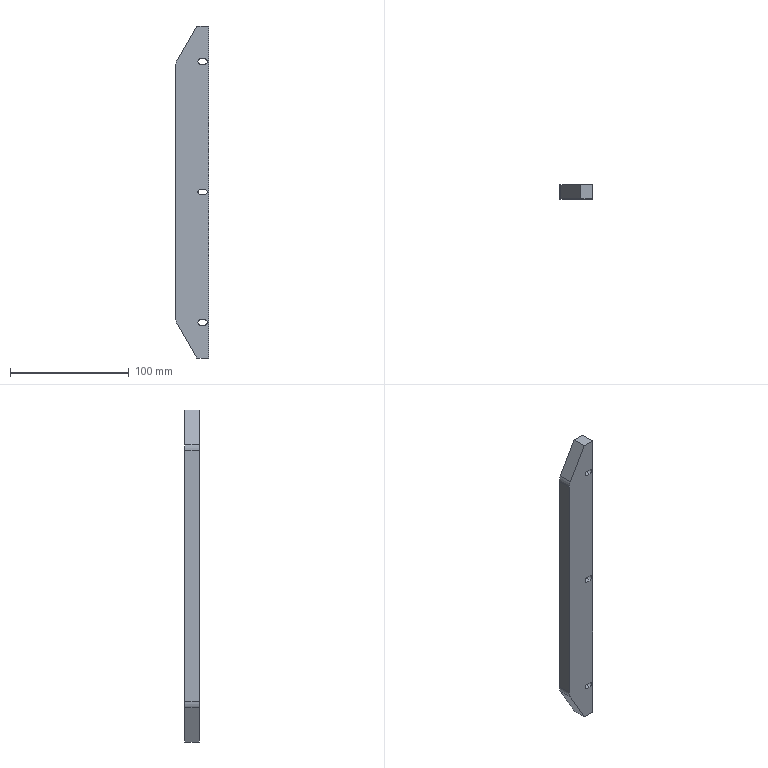Part | STEP file | Tdangtiao-002_デフォルト | 1 solid | 34 faces | box 28 x 12 x 280 mm | volume 85542 mm3 | plane 23 | cylinder 11 | commonest cylinder face diameters 4.5 x6 8.5 x3 20 x2
STEP:
#1=CARTESIAN_POINT('',(9.439,2.,32.25));
#2=VERTEX_POINT('',#1);
#3=CARTESIAN_POINT('',(5.939,2.,32.25));
#4=VERTEX_POINT('',#3);
#5=CARTESIAN_POINT('',(5.939,2.,32.25));
#6=DIRECTION('',(-1.,0.,0.));
#7=VECTOR('',#6,1000.);
#8=LINE('',#5,#7);
#9=EDGE_CURVE('',#2,#4,#8,.T.);
#10=ORIENTED_EDGE('',*,*,#9,.F.);
#11=CARTESIAN_POINT('',(9.439,-6.,32.25));
#12=VERTEX_POINT('',#11);
#13=CARTESIAN_POINT('',(9.439,-274.,32.25));
#14=DIRECTION('',(0.,1.,0.));
#15=VECTOR('',#14,1000.);
#16=LINE('',#13,#15);
#17=EDGE_CURVE('',#12,#2,#16,.T.);
#18=ORIENTED_EDGE('',*,*,#17,.F.);
#19=CARTESIAN_POINT('',(5.939,-6.,32.25));
#20=VERTEX_POINT('',#19);
#21=CARTESIAN_POINT('',(-15.311,-6.,32.25));
#22=DIRECTION('',(1.,0.,0.));
#23=VECTOR('',#22,1000.);
#24=LINE('',#21,#23);
#25=EDGE_CURVE('',#20,#12,#24,.T.);
#26=ORIENTED_EDGE('',*,*,#25,.F.);
#27=CARTESIAN_POINT('',(5.939,-274.,32.25));
#28=DIRECTION('',(0.,1.,0.));
#29=VECTOR('',#28,1000.);
#30=LINE('',#27,#29);
#31=EDGE_CURVE('',#20,#4,#30,.T.);
#32=ORIENTED_EDGE('',*,*,#31,.T.);
#33=EDGE_LOOP('',(#10,#18,#26,#32));
#34=FACE_OUTER_BOUND('',#33,.T.);
#35=CARTESIAN_POINT('',(5.939,-274.,32.25));
#36=DIRECTION('',(0.,0.,1.));
#37=DIRECTION('',(1.,0.,0.));
#38=AXIS2_PLACEMENT_3D('',#35,#36,#37);
#39=PLANE('',#38);
#40=ADVANCED_FACE('',(#34),#39,.F.);
#41=CARTESIAN_POINT('',(9.439,2.,27.75));
#42=VERTEX_POINT('',#41);
#43=CARTESIAN_POINT('',(9.439,2.,30.));
#44=DIRECTION('',(0.,-1.,0.));
#45=DIRECTION('',(0.,0.,1.));
#46=AXIS2_PLACEMENT_3D('',#43,#44,#45);
#47=CIRCLE('',#46,2.25);
#48=EDGE_CURVE('',#42,#2,#47,.T.);
#49=ORIENTED_EDGE('',*,*,#48,.F.);
#50=CARTESIAN_POINT('',(9.439,-6.,27.75));
#51=VERTEX_POINT('',#50);
#52=CARTESIAN_POINT('',(9.439,-274.,27.75));
#53=DIRECTION('',(0.,1.,0.));
#54=VECTOR('',#53,1000.);
#55=LINE('',#52,#54);
#56=EDGE_CURVE('',#51,#42,#55,.T.);
#57=ORIENTED_EDGE('',*,*,#56,.F.);
#58=CARTESIAN_POINT('',(9.439,-6.,30.));
#59=DIRECTION('',(0.,1.,0.));
#60=DIRECTION('',(0.,0.,1.));
#61=AXIS2_PLACEMENT_3D('',#58,#59,#60);
#62=CIRCLE('',#61,2.25);
#63=EDGE_CURVE('',#12,#51,#62,.T.);
#64=ORIENTED_EDGE('',*,*,#63,.F.);
#65=ORIENTED_EDGE('',*,*,#17,.T.);
#66=EDGE_LOOP('',(#49,#57,#64,#65));
#67=FACE_OUTER_BOUND('',#66,.T.);
#68=CARTESIAN_POINT('',(9.439,-274.,30.));
#69=DIRECTION('',(0.,1.,0.));
#70=DIRECTION('',(0.,0.,1.));
#71=AXIS2_PLACEMENT_3D('',#68,#69,#70);
#72=CYLINDRICAL_SURFACE('',#71,2.25);
#73=ADVANCED_FACE('',(#67),#72,.F.);
#74=CARTESIAN_POINT('',(5.939,2.,27.75));
#75=VERTEX_POINT('',#74);
#76=CARTESIAN_POINT('',(5.939,2.,27.75));
#77=DIRECTION('',(1.,0.,0.));
#78=VECTOR('',#77,1000.);
#79=LINE('',#76,#78);
#80=EDGE_CURVE('',#75,#42,#79,.T.);
#81=ORIENTED_EDGE('',*,*,#80,.F.);
#82=CARTESIAN_POINT('',(5.939,-6.,27.75));
#83=VERTEX_POINT('',#82);
#84=CARTESIAN_POINT('',(5.939,-274.,27.75));
#85=DIRECTION('',(0.,1.,0.));
#86=VECTOR('',#85,1000.);
#87=LINE('',#84,#86);
#88=EDGE_CURVE('',#83,#75,#87,.T.);
#89=ORIENTED_EDGE('',*,*,#88,.F.);
#90=CARTESIAN_POINT('',(-15.311,-6.,27.75));
#91=DIRECTION('',(-1.,0.,0.));
#92=VECTOR('',#91,1000.);
#93=LINE('',#90,#92);
#94=EDGE_CURVE('',#51,#83,#93,.T.);
#95=ORIENTED_EDGE('',*,*,#94,.F.);
#96=ORIENTED_EDGE('',*,*,#56,.T.);
#97=EDGE_LOOP('',(#81,#89,#95,#96));
#98=FACE_OUTER_BOUND('',#97,.T.);
#99=CARTESIAN_POINT('',(5.939,-274.,27.75));
#100=DIRECTION('',(0.,0.,-1.));
#101=DIRECTION('',(-1.,0.,0.));
#102=AXIS2_PLACEMENT_3D('',#99,#100,#101);
#103=PLANE('',#102);
#104=ADVANCED_FACE('',(#98),#103,.F.);
#105=CARTESIAN_POINT('',(5.939,2.,30.));
#106=DIRECTION('',(0.,-1.,0.));
#107=DIRECTION('',(0.,0.,1.));
#108=AXIS2_PLACEMENT_3D('',#105,#106,#107);
#109=CIRCLE('',#108,2.25);
#110=EDGE_CURVE('',#4,#75,#109,.T.);
#111=ORIENTED_EDGE('',*,*,#110,.F.);
#112=ORIENTED_EDGE('',*,*,#31,.F.);
#113=CARTESIAN_POINT('',(5.939,-6.,30.));
#114=DIRECTION('',(0.,1.,0.));
#115=DIRECTION('',(0.,0.,1.));
#116=AXIS2_PLACEMENT_3D('',#113,#114,#115);
#117=CIRCLE('',#116,2.25);
#118=EDGE_CURVE('',#83,#20,#117,.T.);
#119=ORIENTED_EDGE('',*,*,#118,.F.);
#120=ORIENTED_EDGE('',*,*,#88,.T.);
#121=EDGE_LOOP('',(#111,#112,#119,#120));
#122=FACE_OUTER_BOUND('',#121,.T.);
#123=CARTESIAN_POINT('',(5.939,-274.,30.));
#124=DIRECTION('',(0.,1.,0.));
#125=DIRECTION('',(0.,0.,1.));
#126=AXIS2_PLACEMENT_3D('',#123,#124,#125);
#127=CYLINDRICAL_SURFACE('',#126,2.25);
#128=ADVANCED_FACE('',(#122),#127,.F.);
#129=CARTESIAN_POINT('',(5.939,2.,142.25));
#130=VERTEX_POINT('',#129);
#131=CARTESIAN_POINT('',(5.939,2.,137.75));
#132=VERTEX_POINT('',#131);
#133=CARTESIAN_POINT('',(5.939,2.,140.));
#134=DIRECTION('',(0.,-1.,0.));
#135=DIRECTION('',(0.,0.,1.));
#136=AXIS2_PLACEMENT_3D('',#133,#134,#135);
#137=CIRCLE('',#136,2.25);
#138=EDGE_CURVE('',#130,#132,#137,.T.);
#139=ORIENTED_EDGE('',*,*,#138,.F.);
#140=CARTESIAN_POINT('',(5.939,-6.,142.25));
#141=VERTEX_POINT('',#140);
#142=CARTESIAN_POINT('',(5.939,-274.,142.25));
#143=DIRECTION('',(0.,1.,0.));
#144=VECTOR('',#143,1000.);
#145=LINE('',#142,#144);
#146=EDGE_CURVE('',#141,#130,#145,.T.);
#147=ORIENTED_EDGE('',*,*,#146,.F.);
#148=CARTESIAN_POINT('',(5.939,-6.,137.75));
#149=VERTEX_POINT('',#148);
#150=CARTESIAN_POINT('',(5.939,-6.,140.));
#151=DIRECTION('',(0.,1.,0.));
#152=DIRECTION('',(0.,0.,1.));
#153=AXIS2_PLACEMENT_3D('',#150,#151,#152);
#154=CIRCLE('',#153,2.25);
#155=EDGE_CURVE('',#149,#141,#154,.T.);
#156=ORIENTED_EDGE('',*,*,#155,.F.);
#157=CARTESIAN_POINT('',(5.939,-274.,137.75));
#158=DIRECTION('',(0.,1.,0.));
#159=VECTOR('',#158,1000.);
#160=LINE('',#157,#159);
#161=EDGE_CURVE('',#149,#132,#160,.T.);
#162=ORIENTED_EDGE('',*,*,#161,.T.);
#163=EDGE_LOOP('',(#139,#147,#156,#162));
#164=FACE_OUTER_BOUND('',#163,.T.);
#165=CARTESIAN_POINT('',(5.939,-274.,140.));
#166=DIRECTION('',(0.,1.,0.));
#167=DIRECTION('',(0.,0.,1.));
#168=AXIS2_PLACEMENT_3D('',#165,#166,#167);
#169=CYLINDRICAL_SURFACE('',#168,2.25);
#170=ADVANCED_FACE('',(#164),#169,.F.);
#171=CARTESIAN_POINT('',(9.439,2.,137.75));
#172=VERTEX_POINT('',#171);
#173=CARTESIAN_POINT('',(5.939,2.,137.75));
#174=DIRECTION('',(1.,0.,0.));
#175=VECTOR('',#174,1000.);
#176=LINE('',#173,#175);
#177=EDGE_CURVE('',#132,#172,#176,.T.);
#178=ORIENTED_EDGE('',*,*,#177,.F.);
#179=ORIENTED_EDGE('',*,*,#161,.F.);
#180=CARTESIAN_POINT('',(9.439,-6.,137.75));
#181=VERTEX_POINT('',#180);
#182=CARTESIAN_POINT('',(-15.311,-6.,137.75));
#183=DIRECTION('',(-1.,0.,0.));
#184=VECTOR('',#183,1000.);
#185=LINE('',#182,#184);
#186=EDGE_CURVE('',#181,#149,#185,.T.);
#187=ORIENTED_EDGE('',*,*,#186,.F.);
#188=CARTESIAN_POINT('',(9.439,-274.,137.75));
#189=DIRECTION('',(0.,1.,0.));
#190=VECTOR('',#189,1000.);
#191=LINE('',#188,#190);
#192=EDGE_CURVE('',#181,#172,#191,.T.);
#193=ORIENTED_EDGE('',*,*,#192,.T.);
#194=EDGE_LOOP('',(#178,#179,#187,#193));
#195=FACE_OUTER_BOUND('',#194,.T.);
#196=CARTESIAN_POINT('',(5.939,-274.,137.75));
#197=DIRECTION('',(0.,0.,-1.));
#198=DIRECTION('',(-1.,0.,0.));
#199=AXIS2_PLACEMENT_3D('',#196,#197,#198);
#200=PLANE('',#199);
#201=ADVANCED_FACE('',(#195),#200,.F.);
#202=CARTESIAN_POINT('',(9.439,2.,142.25));
#203=VERTEX_POINT('',#202);
#204=CARTESIAN_POINT('',(9.439,2.,140.));
#205=DIRECTION('',(0.,-1.,0.));
#206=DIRECTION('',(0.,0.,1.));
#207=AXIS2_PLACEMENT_3D('',#204,#205,#206);
#208=CIRCLE('',#207,2.25);
#209=EDGE_CURVE('',#172,#203,#208,.T.);
#210=ORIENTED_EDGE('',*,*,#209,.F.);
#211=ORIENTED_EDGE('',*,*,#192,.F.);
#212=CARTESIAN_POINT('',(9.439,-6.,142.25));
#213=VERTEX_POINT('',#212);
#214=CARTESIAN_POINT('',(9.439,-6.,140.));
#215=DIRECTION('',(0.,1.,0.));
#216=DIRECTION('',(0.,0.,1.));
#217=AXIS2_PLACEMENT_3D('',#214,#215,#216);
#218=CIRCLE('',#217,2.25);
#219=EDGE_CURVE('',#213,#181,#218,.T.);
#220=ORIENTED_EDGE('',*,*,#219,.F.);
#221=CARTESIAN_POINT('',(9.439,-274.,142.25));
#222=DIRECTION('',(0.,1.,0.));
#223=VECTOR('',#222,1000.);
#224=LINE('',#221,#223);
#225=EDGE_CURVE('',#213,#203,#224,.T.);
#226=ORIENTED_EDGE('',*,*,#225,.T.);
#227=EDGE_LOOP('',(#210,#211,#220,#226));
#228=FACE_OUTER_BOUND('',#227,.T.);
#229=CARTESIAN_POINT('',(9.439,-274.,140.));
#230=DIRECTION('',(0.,1.,0.));
#231=DIRECTION('',(0.,0.,1.));
#232=AXIS2_PLACEMENT_3D('',#229,#230,#231);
#233=CYLINDRICAL_SURFACE('',#232,2.25);
#234=ADVANCED_FACE('',(#228),#233,.F.);
#235=CARTESIAN_POINT('',(5.939,2.,142.25));
#236=DIRECTION('',(-1.,0.,0.));
#237=VECTOR('',#236,1000.);
#238=LINE('',#235,#237);
#239=EDGE_CURVE('',#203,#130,#238,.T.);
#240=ORIENTED_EDGE('',*,*,#239,.F.);
#241=ORIENTED_EDGE('',*,*,#225,.F.);
#242=CARTESIAN_POINT('',(-15.311,-6.,142.25));
#243=DIRECTION('',(1.,0.,0.));
#244=VECTOR('',#243,1000.);
#245=LINE('',#242,#244);
#246=EDGE_CURVE('',#141,#213,#245,.T.);
#247=ORIENTED_EDGE('',*,*,#246,.F.);
#248=ORIENTED_EDGE('',*,*,#146,.T.);
#249=EDGE_LOOP('',(#240,#241,#247,#248));
#250=FACE_OUTER_BOUND('',#249,.T.);
#251=CARTESIAN_POINT('',(5.939,-274.,142.25));
#252=DIRECTION('',(0.,0.,1.));
#253=DIRECTION('',(1.,0.,0.));
#254=AXIS2_PLACEMENT_3D('',#251,#252,#253);
#255=PLANE('',#254);
#256=ADVANCED_FACE('',(#250),#255,.F.);
#257=CARTESIAN_POINT('',(5.939,2.,252.25));
#258=VERTEX_POINT('',#257);
#259=CARTESIAN_POINT('',(5.939,2.,247.75));
#260=VERTEX_POINT('',#259);
#261=CARTESIAN_POINT('',(5.939,2.,250.));
#262=DIRECTION('',(0.,-1.,0.));
#263=DIRECTION('',(0.,0.,1.));
#264=AXIS2_PLACEMENT_3D('',#261,#262,#263);
#265=CIRCLE('',#264,2.25);
#266=EDGE_CURVE('',#258,#260,#265,.T.);
#267=ORIENTED_EDGE('',*,*,#266,.F.);
#268=CARTESIAN_POINT('',(5.939,-6.,252.25));
#269=VERTEX_POINT('',#268);
#270=CARTESIAN_POINT('',(5.939,-274.,252.25));
#271=DIRECTION('',(0.,1.,0.));
#272=VECTOR('',#271,1000.);
#273=LINE('',#270,#272);
#274=EDGE_CURVE('',#269,#258,#273,.T.);
#275=ORIENTED_EDGE('',*,*,#274,.F.);
#276=CARTESIAN_POINT('',(5.939,-6.,247.75));
#277=VERTEX_POINT('',#276);
#278=CARTESIAN_POINT('',(5.939,-6.,250.));
#279=DIRECTION('',(0.,1.,0.));
#280=DIRECTION('',(0.,0.,1.));
#281=AXIS2_PLACEMENT_3D('',#278,#279,#280);
#282=CIRCLE('',#281,2.25);
#283=EDGE_CURVE('',#277,#269,#282,.T.);
#284=ORIENTED_EDGE('',*,*,#283,.F.);
#285=CARTESIAN_POINT('',(5.939,-274.,247.75));
#286=DIRECTION('',(0.,1.,0.));
#287=VECTOR('',#286,1000.);
#288=LINE('',#285,#287);
#289=EDGE_CURVE('',#277,#260,#288,.T.);
#290=ORIENTED_EDGE('',*,*,#289,.T.);
#291=EDGE_LOOP('',(#267,#275,#284,#290));
#292=FACE_OUTER_BOUND('',#291,.T.);
#293=CARTESIAN_POINT('',(5.939,-274.,250.));
#294=DIRECTION('',(0.,1.,0.));
#295=DIRECTION('',(0.,0.,1.));
#296=AXIS2_PLACEMENT_3D('',#293,#294,#295);
#297=CYLINDRICAL_SURFACE('',#296,2.25);
#298=ADVANCED_FACE('',(#292),#297,.F.);
#299=CARTESIAN_POINT('',(9.439,2.,247.75));
#300=VERTEX_POINT('',#299);
#301=CARTESIAN_POINT('',(5.939,2.,247.75));
#302=DIRECTION('',(1.,0.,0.));
#303=VECTOR('',#302,1000.);
#304=LINE('',#301,#303);
#305=EDGE_CURVE('',#260,#300,#304,.T.);
#306=ORIENTED_EDGE('',*,*,#305,.F.);
#307=ORIENTED_EDGE('',*,*,#289,.F.);
#308=CARTESIAN_POINT('',(9.439,-6.,247.75));
#309=VERTEX_POINT('',#308);
#310=CARTESIAN_POINT('',(-15.311,-6.,247.75));
#311=DIRECTION('',(-1.,0.,0.));
#312=VECTOR('',#311,1000.);
#313=LINE('',#310,#312);
#314=EDGE_CURVE('',#309,#277,#313,.T.);
#315=ORIENTED_EDGE('',*,*,#314,.F.);
#316=CARTESIAN_POINT('',(9.439,-274.,247.75));
#317=DIRECTION('',(0.,1.,0.));
#318=VECTOR('',#317,1000.);
#319=LINE('',#316,#318);
#320=EDGE_CURVE('',#309,#300,#319,.T.);
#321=ORIENTED_EDGE('',*,*,#320,.T.);
#322=EDGE_LOOP('',(#306,#307,#315,#321));
#323=FACE_OUTER_BOUND('',#322,.T.);
#324=CARTESIAN_POINT('',(5.939,-274.,247.75));
#325=DIRECTION('',(0.,0.,-1.));
#326=DIRECTION('',(-1.,0.,0.));
#327=AXIS2_PLACEMENT_3D('',#324,#325,#326);
#328=PLANE('',#327);
#329=ADVANCED_FACE('',(#323),#328,.F.);
#330=CARTESIAN_POINT('',(9.439,2.,252.25));
#331=VERTEX_POINT('',#330);
#332=CARTESIAN_POINT('',(9.439,2.,250.));
#333=DIRECTION('',(0.,-1.,0.));
#334=DIRECTION('',(0.,0.,1.));
#335=AXIS2_PLACEMENT_3D('',#332,#333,#334);
#336=CIRCLE('',#335,2.25);
#337=EDGE_CURVE('',#300,#331,#336,.T.);
#338=ORIENTED_EDGE('',*,*,#337,.F.);
#339=ORIENTED_EDGE('',*,*,#320,.F.);
#340=CARTESIAN_POINT('',(9.439,-6.,252.25));
#341=VERTEX_POINT('',#340);
#342=CARTESIAN_POINT('',(9.439,-6.,250.));
#343=DIRECTION('',(0.,1.,0.));
#344=DIRECTION('',(0.,0.,1.));
#345=AXIS2_PLACEMENT_3D('',#342,#343,#344);
#346=CIRCLE('',#345,2.25);
#347=EDGE_CURVE('',#341,#309,#346,.T.);
#348=ORIENTED_EDGE('',*,*,#347,.F.);
#349=CARTESIAN_POINT('',(9.439,-274.,252.25));
#350=DIRECTION('',(0.,1.,0.));
#351=VECTOR('',#350,1000.);
#352=LINE('',#349,#351);
#353=EDGE_CURVE('',#341,#331,#352,.T.);
#354=ORIENTED_EDGE('',*,*,#353,.T.);
#355=EDGE_LOOP('',(#338,#339,#348,#354));
#356=FACE_OUTER_BOUND('',#355,.T.);
#357=CARTESIAN_POINT('',(9.439,-274.,250.));
#358=DIRECTION('',(0.,1.,0.));
#359=DIRECTION('',(0.,0.,1.));
#360=AXIS2_PLACEMENT_3D('',#357,#358,#359);
#361=CYLINDRICAL_SURFACE('',#360,2.25);
#362=ADVANCED_FACE('',(#356),#361,.F.);
#363=CARTESIAN_POINT('',(5.939,2.,252.25));
#364=DIRECTION('',(-1.,0.,0.));
#365=VECTOR('',#364,1000.);
#366=LINE('',#363,#365);
#367=EDGE_CURVE('',#331,#258,#366,.T.);
#368=ORIENTED_EDGE('',*,*,#367,.F.);
#369=ORIENTED_EDGE('',*,*,#353,.F.);
#370=CARTESIAN_POINT('',(-15.311,-6.,252.25));
#371=DIRECTION('',(1.,0.,0.));
#372=VECTOR('',#371,1000.);
#373=LINE('',#370,#372);
#374=EDGE_CURVE('',#269,#341,#373,.T.);
#375=ORIENTED_EDGE('',*,*,#374,.F.);
#376=ORIENTED_EDGE('',*,*,#274,.T.);
#377=EDGE_LOOP('',(#368,#369,#375,#376));
#378=FACE_OUTER_BOUND('',#377,.T.);
#379=CARTESIAN_POINT('',(5.939,-274.,252.25));
#380=DIRECTION('',(0.,0.,1.));
#381=DIRECTION('',(1.,0.,0.));
#382=AXIS2_PLACEMENT_3D('',#379,#380,#381);
#383=PLANE('',#382);
#384=ADVANCED_FACE('',(#378),#383,.F.);
#385=CARTESIAN_POINT('',(12.689,2.,34.25));
#386=VERTEX_POINT('',#385);
#387=CARTESIAN_POINT('',(12.689,2.,25.75));
#388=VERTEX_POINT('',#387);
#389=CARTESIAN_POINT('',(12.689,2.,280.));
#390=DIRECTION('',(0.,0.,-1.));
#391=VECTOR('',#390,1000.);
#392=LINE('',#389,#391);
#393=EDGE_CURVE('',#386,#388,#392,.T.);
#394=ORIENTED_EDGE('',*,*,#393,.F.);
#395=CARTESIAN_POINT('',(12.689,6.,34.25));
#396=VERTEX_POINT('',#395);
#397=CARTESIAN_POINT('',(12.689,6.,34.25));
#398=DIRECTION('',(0.,1.,0.));
#399=VECTOR('',#398,1000.);
#400=LINE('',#397,#399);
#401=EDGE_CURVE('',#386,#396,#400,.T.);
#402=ORIENTED_EDGE('',*,*,#401,.T.);
#403=CARTESIAN_POINT('',(12.689,6.,135.75));
#404=VERTEX_POINT('',#403);
#405=CARTESIAN_POINT('',(12.689,6.,280.));
#406=DIRECTION('',(0.,0.,-1.));
#407=VECTOR('',#406,1000.);
#408=LINE('',#405,#407);
#409=EDGE_CURVE('',#404,#396,#408,.T.);
#410=ORIENTED_EDGE('',*,*,#409,.F.);
#411=CARTESIAN_POINT('',(12.689,2.,135.75));
#412=VERTEX_POINT('',#411);
#413=CARTESIAN_POINT('',(12.689,6.,135.75));
#414=DIRECTION('',(0.,-1.,0.));
#415=VECTOR('',#414,1000.);
#416=LINE('',#413,#415);
#417=EDGE_CURVE('',#404,#412,#416,.T.);
#418=ORIENTED_EDGE('',*,*,#417,.T.);
#419=CARTESIAN_POINT('',(12.689,2.,144.25));
#420=VERTEX_POINT('',#419);
#421=CARTESIAN_POINT('',(12.689,2.,280.));
#422=DIRECTION('',(0.,0.,-1.));
#423=VECTOR('',#422,1000.);
#424=LINE('',#421,#423);
#425=EDGE_CURVE('',#420,#412,#424,.T.);
#426=ORIENTED_EDGE('',*,*,#425,.F.);
#427=CARTESIAN_POINT('',(12.689,6.,144.25));
#428=VERTEX_POINT('',#427);
#429=CARTESIAN_POINT('',(12.689,6.,144.25));
#430=DIRECTION('',(0.,1.,0.));
#431=VECTOR('',#430,1000.);
#432=LINE('',#429,#431);
#433=EDGE_CURVE('',#420,#428,#432,.T.);
#434=ORIENTED_EDGE('',*,*,#433,.T.);
#435=CARTESIAN_POINT('',(12.689,6.,245.75));
#436=VERTEX_POINT('',#435);
#437=CARTESIAN_POINT('',(12.689,6.,280.));
#438=DIRECTION('',(0.,0.,-1.));
#439=VECTOR('',#438,1000.);
#440=LINE('',#437,#439);
#441=EDGE_CURVE('',#436,#428,#440,.T.);
#442=ORIENTED_EDGE('',*,*,#441,.F.);
#443=CARTESIAN_POINT('',(12.689,2.,245.75));
#444=VERTEX_POINT('',#443);
#445=CARTESIAN_POINT('',(12.689,6.,245.75));
#446=DIRECTION('',(0.,-1.,0.));
#447=VECTOR('',#446,1000.);
#448=LINE('',#445,#447);
#449=EDGE_CURVE('',#436,#444,#448,.T.);
#450=ORIENTED_EDGE('',*,*,#449,.T.);
#451=CARTESIAN_POINT('',(12.689,2.,254.25));
#452=VERTEX_POINT('',#451);
#453=CARTESIAN_POINT('',(12.689,2.,280.));
#454=DIRECTION('',(0.,0.,-1.));
#455=VECTOR('',#454,1000.);
#456=LINE('',#453,#455);
#457=EDGE_CURVE('',#452,#444,#456,.T.);
#458=ORIENTED_EDGE('',*,*,#457,.F.);
#459=CARTESIAN_POINT('',(12.689,6.,254.25));
#460=VERTEX_POINT('',#459);
#461=CARTESIAN_POINT('',(12.689,6.,254.25));
#462=DIRECTION('',(0.,1.,0.));
#463=VECTOR('',#462,1000.);
#464=LINE('',#461,#463);
#465=EDGE_CURVE('',#452,#460,#464,.T.);
#466=ORIENTED_EDGE('',*,*,#465,.T.);
#467=CARTESIAN_POINT('',(12.689,6.,280.));
#468=VERTEX_POINT('',#467);
#469=CARTESIAN_POINT('',(12.689,6.,280.));
#470=DIRECTION('',(0.,0.,-1.));
#471=VECTOR('',#470,1000.);
#472=LINE('',#469,#471);
#473=EDGE_CURVE('',#468,#460,#472,.T.);
#474=ORIENTED_EDGE('',*,*,#473,.F.);
#475=CARTESIAN_POINT('',(12.689,-6.,280.));
#476=VERTEX_POINT('',#475);
#477=CARTESIAN_POINT('',(12.689,6.,280.));
#478=DIRECTION('',(0.,1.,0.));
#479=VECTOR('',#478,1000.);
#480=LINE('',#477,#479);
#481=EDGE_CURVE('',#476,#468,#480,.T.);
#482=ORIENTED_EDGE('',*,*,#481,.F.);
#483=CARTESIAN_POINT('',(12.689,-6.,0.));
#484=VERTEX_POINT('',#483);
#485=CARTESIAN_POINT('',(12.689,-6.,280.));
#486=DIRECTION('',(0.,0.,-1.));
#487=VECTOR('',#486,1000.);
#488=LINE('',#485,#487);
#489=EDGE_CURVE('',#476,#484,#488,.T.);
#490=ORIENTED_EDGE('',*,*,#489,.T.);
#491=CARTESIAN_POINT('',(12.689,6.,0.));
#492=VERTEX_POINT('',#491);
#493=CARTESIAN_POINT('',(12.689,6.,0.));
#494=DIRECTION('',(0.,1.,0.));
#495=VECTOR('',#494,1000.);
#496=LINE('',#493,#495);
#497=EDGE_CURVE('',#484,#492,#496,.T.);
#498=ORIENTED_EDGE('',*,*,#497,.T.);
#499=CARTESIAN_POINT('',(12.689,6.,25.75));
#500=VERTEX_POINT('',#499);
#501=CARTESIAN_POINT('',(12.689,6.,280.));
#502=DIRECTION('',(0.,0.,-1.));
#503=VECTOR('',#502,1000.);
#504=LINE('',#501,#503);
#505=EDGE_CURVE('',#500,#492,#504,.T.);
#506=ORIENTED_EDGE('',*,*,#505,.F.);
#507=CARTESIAN_POINT('',(12.689,6.,25.75));
#508=DIRECTION('',(0.,-1.,0.));
#509=VECTOR('',#508,1000.);
#510=LINE('',#507,#509);
#511=EDGE_CURVE('',#500,#388,#510,.T.);
#512=ORIENTED_EDGE('',*,*,#511,.T.);
#513=EDGE_LOOP('',(#394,#402,#410,#418,#426,#434,#442,#450,#458,#466,#474,#482,#490,#498,#506,#512));
#514=FACE_OUTER_BOUND('',#513,.T.);
#515=CARTESIAN_POINT('',(12.689,6.,280.));
#516=DIRECTION('',(-1.,0.,0.));
#517=DIRECTION('',(0.,-1.,0.));
#518=AXIS2_PLACEMENT_3D('',#515,#516,#517);
#519=PLANE('',#518);
#520=ADVANCED_FACE('',(#514),#519,.F.);
#521=CARTESIAN_POINT('',(-15.311,6.,246.144));
#522=VERTEX_POINT('',#521);
#523=CARTESIAN_POINT('',(-15.311,6.,33.856));
#524=VERTEX_POINT('',#523);
#525=CARTESIAN_POINT('',(-15.311,6.,280.));
#526=DIRECTION('',(0.,0.,-1.));
#527=VECTOR('',#526,1000.);
#528=LINE('',#525,#527);
#529=EDGE_CURVE('',#522,#524,#528,.T.);
#530=ORIENTED_EDGE('',*,*,#529,.F.);
#531=CARTESIAN_POINT('',(-13.971,6.,251.144));
#532=VERTEX_POINT('',#531);
#533=CARTESIAN_POINT('',(-5.311,6.,246.144));
#534=DIRECTION('',(0.,1.,0.));
#535=DIRECTION('',(0.,0.,-1.));
#536=AXIS2_PLACEMENT_3D('',#533,#534,#535);
#537=CIRCLE('',#536,10.);
#538=EDGE_CURVE('',#522,#532,#537,.T.);
#539=ORIENTED_EDGE('',*,*,#538,.T.);
#540=CARTESIAN_POINT('',(2.689,6.,280.));
#541=VERTEX_POINT('',#540);
#542=CARTESIAN_POINT('',(2.689,6.,280.));
#543=DIRECTION('',(-0.5,0.,-0.866));
#544=VECTOR('',#543,1000.);
#545=LINE('',#542,#544);
#546=EDGE_CURVE('',#541,#532,#545,.T.);
#547=ORIENTED_EDGE('',*,*,#546,.F.);
#548=CARTESIAN_POINT('',(-15.311,6.,280.));
#549=DIRECTION('',(-1.,0.,0.));
#550=VECTOR('',#549,1000.);
#551=LINE('',#548,#550);
#552=EDGE_CURVE('',#468,#541,#551,.T.);
#553=ORIENTED_EDGE('',*,*,#552,.F.);
#554=ORIENTED_EDGE('',*,*,#473,.T.);
#555=CARTESIAN_POINT('',(5.939,6.,254.25));
#556=VERTEX_POINT('',#555);
#557=CARTESIAN_POINT('',(23.402,6.,254.25));
#558=DIRECTION('',(1.,0.,0.));
#559=VECTOR('',#558,1000.);
#560=LINE('',#557,#559);
#561=EDGE_CURVE('',#556,#460,#560,.T.);
#562=ORIENTED_EDGE('',*,*,#561,.F.);
#563=CARTESIAN_POINT('',(5.939,6.,245.75));
#564=VERTEX_POINT('',#563);
#565=CARTESIAN_POINT('',(5.939,6.,250.));
#566=DIRECTION('',(0.,1.,0.));
#567=DIRECTION('',(0.,0.,1.));
#568=AXIS2_PLACEMENT_3D('',#565,#566,#567);
#569=CIRCLE('',#568,4.25);
#570=EDGE_CURVE('',#564,#556,#569,.T.);
#571=ORIENTED_EDGE('',*,*,#570,.F.);
#572=CARTESIAN_POINT('',(9.439,6.,245.75));
#573=DIRECTION('',(-1.,0.,0.));
#574=VECTOR('',#573,1000.);
#575=LINE('',#572,#574);
#576=EDGE_CURVE('',#436,#564,#575,.T.);
#577=ORIENTED_EDGE('',*,*,#576,.F.);
#578=ORIENTED_EDGE('',*,*,#441,.T.);
#579=CARTESIAN_POINT('',(5.939,6.,144.25));
#580=VERTEX_POINT('',#579);
#581=CARTESIAN_POINT('',(23.402,6.,144.25));
#582=DIRECTION('',(1.,0.,0.));
#583=VECTOR('',#582,1000.);
#584=LINE('',#581,#583);
#585=EDGE_CURVE('',#580,#428,#584,.T.);
#586=ORIENTED_EDGE('',*,*,#585,.F.);
#587=CARTESIAN_POINT('',(5.939,6.,135.75));
#588=VERTEX_POINT('',#587);
#589=CARTESIAN_POINT('',(5.939,6.,140.));
#590=DIRECTION('',(0.,1.,0.));
#591=DIRECTION('',(0.,0.,1.));
#592=AXIS2_PLACEMENT_3D('',#589,#590,#591);
#593=CIRCLE('',#592,4.25);
#594=EDGE_CURVE('',#588,#580,#593,.T.);
#595=ORIENTED_EDGE('',*,*,#594,.F.);
#596=CARTESIAN_POINT('',(9.439,6.,135.75));
#597=DIRECTION('',(-1.,0.,0.));
#598=VECTOR('',#597,1000.);
#599=LINE('',#596,#598);
#600=EDGE_CURVE('',#404,#588,#599,.T.);
#601=ORIENTED_EDGE('',*,*,#600,.F.);
#602=ORIENTED_EDGE('',*,*,#409,.T.);
#603=CARTESIAN_POINT('',(5.939,6.,34.25));
#604=VERTEX_POINT('',#603);
#605=CARTESIAN_POINT('',(23.402,6.,34.25));
#606=DIRECTION('',(1.,0.,0.));
#607=VECTOR('',#606,1000.);
#608=LINE('',#605,#607);
#609=EDGE_CURVE('',#604,#396,#608,.T.);
#610=ORIENTED_EDGE('',*,*,#609,.F.);
#611=CARTESIAN_POINT('',(5.939,6.,25.75));
#612=VERTEX_POINT('',#611);
#613=CARTESIAN_POINT('',(5.939,6.,30.));
#614=DIRECTION('',(0.,1.,0.));
#615=DIRECTION('',(0.,0.,1.));
#616=AXIS2_PLACEMENT_3D('',#613,#614,#615);
#617=CIRCLE('',#616,4.25);
#618=EDGE_CURVE('',#612,#604,#617,.T.);
#619=ORIENTED_EDGE('',*,*,#618,.F.);
#620=CARTESIAN_POINT('',(9.439,6.,25.75));
#621=DIRECTION('',(-1.,0.,0.));
#622=VECTOR('',#621,1000.);
#623=LINE('',#620,#622);
#624=EDGE_CURVE('',#500,#612,#623,.T.);
#625=ORIENTED_EDGE('',*,*,#624,.F.);
#626=ORIENTED_EDGE('',*,*,#505,.T.);
#627=CARTESIAN_POINT('',(2.689,6.,0.));
#628=VERTEX_POINT('',#627);
#629=CARTESIAN_POINT('',(-15.311,6.,0.));
#630=DIRECTION('',(-1.,0.,0.));
#631=VECTOR('',#630,1000.);
#632=LINE('',#629,#631);
#633=EDGE_CURVE('',#492,#628,#632,.T.);
#634=ORIENTED_EDGE('',*,*,#633,.T.);
#635=CARTESIAN_POINT('',(-13.971,6.,28.856));
#636=VERTEX_POINT('',#635);
#637=CARTESIAN_POINT('',(2.689,6.,0.));
#638=DIRECTION('',(0.5,0.,-0.866));
#639=VECTOR('',#638,1000.);
#640=LINE('',#637,#639);
#641=EDGE_CURVE('',#636,#628,#640,.T.);
#642=ORIENTED_EDGE('',*,*,#641,.F.);
#643=CARTESIAN_POINT('',(-5.311,6.,33.856));
#644=DIRECTION('',(0.,1.,0.));
#645=DIRECTION('',(0.,0.,-1.));
#646=AXIS2_PLACEMENT_3D('',#643,#644,#645);
#647=CIRCLE('',#646,10.);
#648=EDGE_CURVE('',#636,#524,#647,.T.);
#649=ORIENTED_EDGE('',*,*,#648,.T.);
#650=EDGE_LOOP('',(#530,#539,#547,#553,#554,#562,#571,#577,#578,#586,#595,#601,#602,#610,#619,#625,#626,#634,#642,#649));
#651=FACE_OUTER_BOUND('',#650,.T.);
#652=CARTESIAN_POINT('',(-15.311,6.,280.));
#653=DIRECTION('',(0.,-1.,0.));
#654=DIRECTION('',(0.,0.,-1.));
#655=AXIS2_PLACEMENT_3D('',#652,#653,#654);
#656=PLANE('',#655);
#657=ADVANCED_FACE('',(#651),#656,.F.);
#658=CARTESIAN_POINT('',(-15.311,-6.,246.144));
#659=VERTEX_POINT('',#658);
#660=CARTESIAN_POINT('',(-15.311,-6.,33.856));
#661=VERTEX_POINT('',#660);
#662=CARTESIAN_POINT('',(-15.311,-6.,280.));
#663=DIRECTION('',(0.,0.,-1.));
#664=VECTOR('',#663,1000.);
#665=LINE('',#662,#664);
#666=EDGE_CURVE('',#659,#661,#665,.T.);
#667=ORIENTED_EDGE('',*,*,#666,.F.);
#668=CARTESIAN_POINT('',(-15.311,6.,246.144));
#669=DIRECTION('',(0.,1.,0.));
#670=VECTOR('',#669,1000.);
#671=LINE('',#668,#670);
#672=EDGE_CURVE('',#659,#522,#671,.T.);
#673=ORIENTED_EDGE('',*,*,#672,.T.);
#674=ORIENTED_EDGE('',*,*,#529,.T.);
#675=CARTESIAN_POINT('',(-15.311,6.,33.856));
#676=DIRECTION('',(0.,-1.,0.));
#677=VECTOR('',#676,1000.);
#678=LINE('',#675,#677);
#679=EDGE_CURVE('',#524,#661,#678,.T.);
#680=ORIENTED_EDGE('',*,*,#679,.T.);
#681=EDGE_LOOP('',(#667,#673,#674,#680));
#682=FACE_OUTER_BOUND('',#681,.T.);
#683=CARTESIAN_POINT('',(-15.311,6.,280.));
#684=DIRECTION('',(1.,0.,0.));
#685=DIRECTION('',(0.,1.,0.));
#686=AXIS2_PLACEMENT_3D('',#683,#684,#685);
#687=PLANE('',#686);
#688=ADVANCED_FACE('',(#682),#687,.F.);
#689=ORIENTED_EDGE('',*,*,#186,.T.);
#690=ORIENTED_EDGE('',*,*,#155,.T.);
#691=ORIENTED_EDGE('',*,*,#246,.T.);
#692=ORIENTED_EDGE('',*,*,#219,.T.);
#693=EDGE_LOOP('',(#689,#690,#691,#692));
#694=FACE_BOUND('',#693,.T.);
#695=ORIENTED_EDGE('',*,*,#314,.T.);
#696=ORIENTED_EDGE('',*,*,#283,.T.);
#697=ORIENTED_EDGE('',*,*,#374,.T.);
#698=ORIENTED_EDGE('',*,*,#347,.T.);
#699=EDGE_LOOP('',(#695,#696,#697,#698));
#700=FACE_BOUND('',#699,.T.);
#701=CARTESIAN_POINT('',(2.689,-6.,280.));
#702=VERTEX_POINT('',#701);
#703=CARTESIAN_POINT('',(-13.971,-6.,251.144));
#704=VERTEX_POINT('',#703);
#705=CARTESIAN_POINT('',(-1.811,-6.,272.206));
#706=DIRECTION('',(-0.5,0.,-0.866));
#707=VECTOR('',#706,1000.);
#708=LINE('',#705,#707);
#709=EDGE_CURVE('',#702,#704,#708,.T.);
#710=ORIENTED_EDGE('',*,*,#709,.T.);
#711=CARTESIAN_POINT('',(-5.311,-6.,246.144));
#712=DIRECTION('',(0.,-1.,0.));
#713=DIRECTION('',(0.,0.,1.));
#714=AXIS2_PLACEMENT_3D('',#711,#712,#713);
#715=CIRCLE('',#714,10.);
#716=EDGE_CURVE('',#704,#659,#715,.T.);
#717=ORIENTED_EDGE('',*,*,#716,.T.);
#718=ORIENTED_EDGE('',*,*,#666,.T.);
#719=CARTESIAN_POINT('',(-13.971,-6.,28.856));
#720=VERTEX_POINT('',#719);
#721=CARTESIAN_POINT('',(-5.311,-6.,33.856));
#722=DIRECTION('',(0.,-1.,0.));
#723=DIRECTION('',(0.,0.,1.));
#724=AXIS2_PLACEMENT_3D('',#721,#722,#723);
#725=CIRCLE('',#724,10.);
#726=EDGE_CURVE('',#661,#720,#725,.T.);
#727=ORIENTED_EDGE('',*,*,#726,.T.);
#728=CARTESIAN_POINT('',(2.689,-6.,0.));
#729=VERTEX_POINT('',#728);
#730=CARTESIAN_POINT('',(-123.055,-6.,217.794));
#731=DIRECTION('',(0.5,0.,-0.866));
#732=VECTOR('',#731,1000.);
#733=LINE('',#730,#732);
#734=EDGE_CURVE('',#720,#729,#733,.T.);
#735=ORIENTED_EDGE('',*,*,#734,.T.);
#736=CARTESIAN_POINT('',(-15.311,-6.,0.));
#737=DIRECTION('',(1.,0.,0.));
#738=VECTOR('',#737,1000.);
#739=LINE('',#736,#738);
#740=EDGE_CURVE('',#729,#484,#739,.T.);
#741=ORIENTED_EDGE('',*,*,#740,.T.);
#742=ORIENTED_EDGE('',*,*,#489,.F.);
#743=CARTESIAN_POINT('',(-15.311,-6.,280.));
#744=DIRECTION('',(1.,0.,0.));
#745=VECTOR('',#744,1000.);
#746=LINE('',#743,#745);
#747=EDGE_CURVE('',#702,#476,#746,.T.);
#748=ORIENTED_EDGE('',*,*,#747,.F.);
#749=EDGE_LOOP('',(#710,#717,#718,#727,#735,#741,#742,#748));
#750=FACE_OUTER_BOUND('',#749,.T.);
#751=ORIENTED_EDGE('',*,*,#118,.T.);
#752=ORIENTED_EDGE('',*,*,#25,.T.);
#753=ORIENTED_EDGE('',*,*,#63,.T.);
#754=ORIENTED_EDGE('',*,*,#94,.T.);
#755=EDGE_LOOP('',(#751,#752,#753,#754));
#756=FACE_BOUND('',#755,.T.);
#757=CARTESIAN_POINT('',(-15.311,-6.,280.));
#758=DIRECTION('',(0.,1.,0.));
#759=DIRECTION('',(0.,0.,1.));
#760=AXIS2_PLACEMENT_3D('',#757,#758,#759);
#761=PLANE('',#760);
#762=ADVANCED_FACE('',(#694,#700,#750,#756),#761,.F.);
#763=CARTESIAN_POINT('',(2.689,0.,280.));
#764=DIRECTION('',(0.,1.,0.));
#765=VECTOR('',#764,1000.);
#766=LINE('',#763,#765);
#767=EDGE_CURVE('',#702,#541,#766,.T.);
#768=ORIENTED_EDGE('',*,*,#767,.F.);
#769=ORIENTED_EDGE('',*,*,#747,.T.);
#770=ORIENTED_EDGE('',*,*,#481,.T.);
#771=ORIENTED_EDGE('',*,*,#552,.T.);
#772=EDGE_LOOP('',(#768,#769,#770,#771));
#773=FACE_OUTER_BOUND('',#772,.T.);
#774=CARTESIAN_POINT('',(0.,0.,280.));
#775=DIRECTION('',(0.,0.,1.));
#776=DIRECTION('',(1.,0.,0.));
#777=AXIS2_PLACEMENT_3D('',#774,#775,#776);
#778=PLANE('',#777);
#779=ADVANCED_FACE('',(#773),#778,.T.);
#780=ORIENTED_EDGE('',*,*,#740,.F.);
#781=CARTESIAN_POINT('',(2.689,0.,0.));
#782=DIRECTION('',(0.,1.,0.));
#783=VECTOR('',#782,1000.);
#784=LINE('',#781,#783);
#785=EDGE_CURVE('',#729,#628,#784,.T.);
#786=ORIENTED_EDGE('',*,*,#785,.T.);
#787=ORIENTED_EDGE('',*,*,#633,.F.);
#788=ORIENTED_EDGE('',*,*,#497,.F.);
#789=EDGE_LOOP('',(#780,#786,#787,#788));
#790=FACE_OUTER_BOUND('',#789,.T.);
#791=CARTESIAN_POINT('',(0.,0.,0.));
#792=DIRECTION('',(0.,0.,1.));
#793=DIRECTION('',(1.,0.,0.));
#794=AXIS2_PLACEMENT_3D('',#791,#792,#793);
#795=PLANE('',#794);
#796=ADVANCED_FACE('',(#790),#795,.F.);
#797=CARTESIAN_POINT('',(5.939,2.,254.25));
#798=VERTEX_POINT('',#797);
#799=CARTESIAN_POINT('',(5.939,2.,254.25));
#800=DIRECTION('',(1.,0.,0.));
#801=VECTOR('',#800,1000.);
#802=LINE('',#799,#801);
#803=EDGE_CURVE('',#798,#452,#802,.T.);
#804=ORIENTED_EDGE('',*,*,#803,.F.);
#805=CARTESIAN_POINT('',(5.939,2.,254.25));
#806=DIRECTION('',(0.,1.,0.));
#807=VECTOR('',#806,1000.);
#808=LINE('',#805,#807);
#809=EDGE_CURVE('',#798,#556,#808,.T.);
#810=ORIENTED_EDGE('',*,*,#809,.T.);
#811=ORIENTED_EDGE('',*,*,#561,.T.);
#812=ORIENTED_EDGE('',*,*,#465,.F.);
#813=EDGE_LOOP('',(#804,#810,#811,#812));
#814=FACE_OUTER_BOUND('',#813,.T.);
#815=CARTESIAN_POINT('',(23.402,2.,254.25));
#816=DIRECTION('',(0.,0.,1.));
#817=DIRECTION('',(1.,0.,0.));
#818=AXIS2_PLACEMENT_3D('',#815,#816,#817);
#819=PLANE('',#818);
#820=ADVANCED_FACE('',(#814),#819,.F.);
#821=ORIENTED_EDGE('',*,*,#576,.T.);
#822=CARTESIAN_POINT('',(5.939,2.,245.75));
#823=VERTEX_POINT('',#822);
#824=CARTESIAN_POINT('',(5.939,2.,245.75));
#825=DIRECTION('',(0.,1.,0.));
#826=VECTOR('',#825,1000.);
#827=LINE('',#824,#826);
#828=EDGE_CURVE('',#823,#564,#827,.T.);
#829=ORIENTED_EDGE('',*,*,#828,.F.);
#830=CARTESIAN_POINT('',(9.439,2.,245.75));
#831=DIRECTION('',(-1.,0.,0.));
#832=VECTOR('',#831,1000.);
#833=LINE('',#830,#832);
#834=EDGE_CURVE('',#444,#823,#833,.T.);
#835=ORIENTED_EDGE('',*,*,#834,.F.);
#836=ORIENTED_EDGE('',*,*,#449,.F.);
#837=EDGE_LOOP('',(#821,#829,#835,#836));
#838=FACE_OUTER_BOUND('',#837,.T.);
#839=CARTESIAN_POINT('',(9.439,2.,245.75));
#840=DIRECTION('',(0.,0.,-1.));
#841=DIRECTION('',(-1.,0.,0.));
#842=AXIS2_PLACEMENT_3D('',#839,#840,#841);
#843=PLANE('',#842);
#844=ADVANCED_FACE('',(#838),#843,.F.);
#845=ORIENTED_EDGE('',*,*,#266,.T.);
#846=ORIENTED_EDGE('',*,*,#305,.T.);
#847=ORIENTED_EDGE('',*,*,#337,.T.);
#848=ORIENTED_EDGE('',*,*,#367,.T.);
#849=EDGE_LOOP('',(#845,#846,#847,#848));
#850=FACE_BOUND('',#849,.T.);
#851=ORIENTED_EDGE('',*,*,#457,.T.);
#852=ORIENTED_EDGE('',*,*,#834,.T.);
#853=CARTESIAN_POINT('',(5.939,2.,250.));
#854=DIRECTION('',(0.,1.,0.));
#855=DIRECTION('',(0.,0.,1.));
#856=AXIS2_PLACEMENT_3D('',#853,#854,#855);
#857=CIRCLE('',#856,4.25);
#858=EDGE_CURVE('',#823,#798,#857,.T.);
#859=ORIENTED_EDGE('',*,*,#858,.T.);
#860=ORIENTED_EDGE('',*,*,#803,.T.);
#861=EDGE_LOOP('',(#851,#852,#859,#860));
#862=FACE_OUTER_BOUND('',#861,.T.);
#863=CARTESIAN_POINT('',(5.939,2.,250.));
#864=DIRECTION('',(0.,1.,0.));
#865=DIRECTION('',(0.,0.,1.));
#866=AXIS2_PLACEMENT_3D('',#863,#864,#865);
#867=PLANE('',#866);
#868=ADVANCED_FACE('',(#850,#862),#867,.T.);
#869=ORIENTED_EDGE('',*,*,#570,.T.);
#870=ORIENTED_EDGE('',*,*,#809,.F.);
#871=ORIENTED_EDGE('',*,*,#858,.F.);
#872=ORIENTED_EDGE('',*,*,#828,.T.);
#873=EDGE_LOOP('',(#869,#870,#871,#872));
#874=FACE_OUTER_BOUND('',#873,.T.);
#875=CARTESIAN_POINT('',(5.939,2.,250.));
#876=DIRECTION('',(0.,1.,0.));
#877=DIRECTION('',(0.,0.,1.));
#878=AXIS2_PLACEMENT_3D('',#875,#876,#877);
#879=CYLINDRICAL_SURFACE('',#878,4.25);
#880=ADVANCED_FACE('',(#874),#879,.F.);
#881=CARTESIAN_POINT('',(5.939,2.,144.25));
#882=VERTEX_POINT('',#881);
#883=CARTESIAN_POINT('',(5.939,2.,144.25));
#884=DIRECTION('',(1.,0.,0.));
#885=VECTOR('',#884,1000.);
#886=LINE('',#883,#885);
#887=EDGE_CURVE('',#882,#420,#886,.T.);
#888=ORIENTED_EDGE('',*,*,#887,.F.);
#889=CARTESIAN_POINT('',(5.939,2.,144.25));
#890=DIRECTION('',(0.,1.,0.));
#891=VECTOR('',#890,1000.);
#892=LINE('',#889,#891);
#893=EDGE_CURVE('',#882,#580,#892,.T.);
#894=ORIENTED_EDGE('',*,*,#893,.T.);
#895=ORIENTED_EDGE('',*,*,#585,.T.);
#896=ORIENTED_EDGE('',*,*,#433,.F.);
#897=EDGE_LOOP('',(#888,#894,#895,#896));
#898=FACE_OUTER_BOUND('',#897,.T.);
#899=CARTESIAN_POINT('',(23.402,2.,144.25));
#900=DIRECTION('',(0.,0.,1.));
#901=DIRECTION('',(1.,0.,0.));
#902=AXIS2_PLACEMENT_3D('',#899,#900,#901);
#903=PLANE('',#902);
#904=ADVANCED_FACE('',(#898),#903,.F.);
#905=ORIENTED_EDGE('',*,*,#600,.T.);
#906=CARTESIAN_POINT('',(5.939,2.,135.75));
#907=VERTEX_POINT('',#906);
#908=CARTESIAN_POINT('',(5.939,2.,135.75));
#909=DIRECTION('',(0.,1.,0.));
#910=VECTOR('',#909,1000.);
#911=LINE('',#908,#910);
#912=EDGE_CURVE('',#907,#588,#911,.T.);
#913=ORIENTED_EDGE('',*,*,#912,.F.);
#914=CARTESIAN_POINT('',(9.439,2.,135.75));
#915=DIRECTION('',(-1.,0.,0.));
#916=VECTOR('',#915,1000.);
#917=LINE('',#914,#916);
#918=EDGE_CURVE('',#412,#907,#917,.T.);
#919=ORIENTED_EDGE('',*,*,#918,.F.);
#920=ORIENTED_EDGE('',*,*,#417,.F.);
#921=EDGE_LOOP('',(#905,#913,#919,#920));
#922=FACE_OUTER_BOUND('',#921,.T.);
#923=CARTESIAN_POINT('',(9.439,2.,135.75));
#924=DIRECTION('',(0.,0.,-1.));
#925=DIRECTION('',(-1.,0.,0.));
#926=AXIS2_PLACEMENT_3D('',#923,#924,#925);
#927=PLANE('',#926);
#928=ADVANCED_FACE('',(#922),#927,.F.);
#929=ORIENTED_EDGE('',*,*,#138,.T.);
#930=ORIENTED_EDGE('',*,*,#177,.T.);
#931=ORIENTED_EDGE('',*,*,#209,.T.);
#932=ORIENTED_EDGE('',*,*,#239,.T.);
#933=EDGE_LOOP('',(#929,#930,#931,#932));
#934=FACE_BOUND('',#933,.T.);
#935=ORIENTED_EDGE('',*,*,#425,.T.);
#936=ORIENTED_EDGE('',*,*,#918,.T.);
#937=CARTESIAN_POINT('',(5.939,2.,140.));
#938=DIRECTION('',(0.,1.,0.));
#939=DIRECTION('',(0.,0.,1.));
#940=AXIS2_PLACEMENT_3D('',#937,#938,#939);
#941=CIRCLE('',#940,4.25);
#942=EDGE_CURVE('',#907,#882,#941,.T.);
#943=ORIENTED_EDGE('',*,*,#942,.T.);
#944=ORIENTED_EDGE('',*,*,#887,.T.);
#945=EDGE_LOOP('',(#935,#936,#943,#944));
#946=FACE_OUTER_BOUND('',#945,.T.);
#947=CARTESIAN_POINT('',(5.939,2.,140.));
#948=DIRECTION('',(0.,1.,0.));
#949=DIRECTION('',(0.,0.,1.));
#950=AXIS2_PLACEMENT_3D('',#947,#948,#949);
#951=PLANE('',#950);
#952=ADVANCED_FACE('',(#934,#946),#951,.T.);
#953=ORIENTED_EDGE('',*,*,#594,.T.);
#954=ORIENTED_EDGE('',*,*,#893,.F.);
#955=ORIENTED_EDGE('',*,*,#942,.F.);
#956=ORIENTED_EDGE('',*,*,#912,.T.);
#957=EDGE_LOOP('',(#953,#954,#955,#956));
#958=FACE_OUTER_BOUND('',#957,.T.);
#959=CARTESIAN_POINT('',(5.939,2.,140.));
#960=DIRECTION('',(0.,1.,0.));
#961=DIRECTION('',(0.,0.,1.));
#962=AXIS2_PLACEMENT_3D('',#959,#960,#961);
#963=CYLINDRICAL_SURFACE('',#962,4.25);
#964=ADVANCED_FACE('',(#958),#963,.F.);
#965=CARTESIAN_POINT('',(5.939,2.,34.25));
#966=VERTEX_POINT('',#965);
#967=CARTESIAN_POINT('',(5.939,2.,34.25));
#968=DIRECTION('',(1.,0.,0.));
#969=VECTOR('',#968,1000.);
#970=LINE('',#967,#969);
#971=EDGE_CURVE('',#966,#386,#970,.T.);
#972=ORIENTED_EDGE('',*,*,#971,.F.);
#973=CARTESIAN_POINT('',(5.939,2.,34.25));
#974=DIRECTION('',(0.,1.,0.));
#975=VECTOR('',#974,1000.);
#976=LINE('',#973,#975);
#977=EDGE_CURVE('',#966,#604,#976,.T.);
#978=ORIENTED_EDGE('',*,*,#977,.T.);
#979=ORIENTED_EDGE('',*,*,#609,.T.);
#980=ORIENTED_EDGE('',*,*,#401,.F.);
#981=EDGE_LOOP('',(#972,#978,#979,#980));
#982=FACE_OUTER_BOUND('',#981,.T.);
#983=CARTESIAN_POINT('',(23.402,2.,34.25));
#984=DIRECTION('',(0.,0.,1.));
#985=DIRECTION('',(1.,0.,0.));
#986=AXIS2_PLACEMENT_3D('',#983,#984,#985);
#987=PLANE('',#986);
#988=ADVANCED_FACE('',(#982),#987,.F.);
#989=ORIENTED_EDGE('',*,*,#624,.T.);
#990=CARTESIAN_POINT('',(5.939,2.,25.75));
#991=VERTEX_POINT('',#990);
#992=CARTESIAN_POINT('',(5.939,2.,25.75));
#993=DIRECTION('',(0.,1.,0.));
#994=VECTOR('',#993,1000.);
#995=LINE('',#992,#994);
#996=EDGE_CURVE('',#991,#612,#995,.T.);
#997=ORIENTED_EDGE('',*,*,#996,.F.);
#998=CARTESIAN_POINT('',(9.439,2.,25.75));
#999=DIRECTION('',(-1.,0.,0.));
#1000=VECTOR('',#999,1000.);
#1001=LINE('',#998,#1000);
#1002=EDGE_CURVE('',#388,#991,#1001,.T.);
#1003=ORIENTED_EDGE('',*,*,#1002,.F.);
#1004=ORIENTED_EDGE('',*,*,#511,.F.);
#1005=EDGE_LOOP('',(#989,#997,#1003,#1004));
#1006=FACE_OUTER_BOUND('',#1005,.T.);
#1007=CARTESIAN_POINT('',(9.439,2.,25.75));
#1008=DIRECTION('',(0.,0.,-1.));
#1009=DIRECTION('',(-1.,0.,0.));
#1010=AXIS2_PLACEMENT_3D('',#1007,#1008,#1009);
#1011=PLANE('',#1010);
#1012=ADVANCED_FACE('',(#1006),#1011,.F.);
#1013=ORIENTED_EDGE('',*,*,#9,.T.);
#1014=ORIENTED_EDGE('',*,*,#110,.T.);
#1015=ORIENTED_EDGE('',*,*,#80,.T.);
#1016=ORIENTED_EDGE('',*,*,#48,.T.);
#1017=EDGE_LOOP('',(#1013,#1014,#1015,#1016));
#1018=FACE_BOUND('',#1017,.T.);
#1019=ORIENTED_EDGE('',*,*,#393,.T.);
#1020=ORIENTED_EDGE('',*,*,#1002,.T.);
#1021=CARTESIAN_POINT('',(5.939,2.,30.));
#1022=DIRECTION('',(0.,1.,0.));
#1023=DIRECTION('',(0.,0.,1.));
#1024=AXIS2_PLACEMENT_3D('',#1021,#1022,#1023);
#1025=CIRCLE('',#1024,4.25);
#1026=EDGE_CURVE('',#991,#966,#1025,.T.);
#1027=ORIENTED_EDGE('',*,*,#1026,.T.);
#1028=ORIENTED_EDGE('',*,*,#971,.T.);
#1029=EDGE_LOOP('',(#1019,#1020,#1027,#1028));
#1030=FACE_OUTER_BOUND('',#1029,.T.);
#1031=CARTESIAN_POINT('',(5.939,2.,30.));
#1032=DIRECTION('',(0.,1.,0.));
#1033=DIRECTION('',(0.,0.,1.));
#1034=AXIS2_PLACEMENT_3D('',#1031,#1032,#1033);
#1035=PLANE('',#1034);
#1036=ADVANCED_FACE('',(#1018,#1030),#1035,.T.);
#1037=ORIENTED_EDGE('',*,*,#618,.T.);
#1038=ORIENTED_EDGE('',*,*,#977,.F.);
#1039=ORIENTED_EDGE('',*,*,#1026,.F.);
#1040=ORIENTED_EDGE('',*,*,#996,.T.);
#1041=EDGE_LOOP('',(#1037,#1038,#1039,#1040));
#1042=FACE_OUTER_BOUND('',#1041,.T.);
#1043=CARTESIAN_POINT('',(5.939,2.,30.));
#1044=DIRECTION('',(0.,1.,0.));
#1045=DIRECTION('',(0.,0.,1.));
#1046=AXIS2_PLACEMENT_3D('',#1043,#1044,#1045);
#1047=CYLINDRICAL_SURFACE('',#1046,4.25);
#1048=ADVANCED_FACE('',(#1042),#1047,.F.);
#1049=ORIENTED_EDGE('',*,*,#734,.F.);
#1050=CARTESIAN_POINT('',(-13.971,-107.,28.856));
#1051=DIRECTION('',(0.,1.,0.));
#1052=VECTOR('',#1051,1000.);
#1053=LINE('',#1050,#1052);
#1054=EDGE_CURVE('',#720,#636,#1053,.T.);
#1055=ORIENTED_EDGE('',*,*,#1054,.T.);
#1056=ORIENTED_EDGE('',*,*,#641,.T.);
#1057=ORIENTED_EDGE('',*,*,#785,.F.);
#1058=EDGE_LOOP('',(#1049,#1055,#1056,#1057));
#1059=FACE_OUTER_BOUND('',#1058,.T.);
#1060=CARTESIAN_POINT('',(2.689,-107.,0.));
#1061=DIRECTION('',(0.866,0.,0.5));
#1062=DIRECTION('',(0.5,0.,-0.866));
#1063=AXIS2_PLACEMENT_3D('',#1060,#1061,#1062);
#1064=PLANE('',#1063);
#1065=ADVANCED_FACE('',(#1059),#1064,.F.);
#1066=ORIENTED_EDGE('',*,*,#546,.T.);
#1067=CARTESIAN_POINT('',(-13.971,-107.,251.144));
#1068=DIRECTION('',(0.,-1.,0.));
#1069=VECTOR('',#1068,1000.);
#1070=LINE('',#1067,#1069);
#1071=EDGE_CURVE('',#532,#704,#1070,.T.);
#1072=ORIENTED_EDGE('',*,*,#1071,.T.);
#1073=ORIENTED_EDGE('',*,*,#709,.F.);
#1074=ORIENTED_EDGE('',*,*,#767,.T.);
#1075=EDGE_LOOP('',(#1066,#1072,#1073,#1074));
#1076=FACE_OUTER_BOUND('',#1075,.T.);
#1077=CARTESIAN_POINT('',(2.689,-107.,280.));
#1078=DIRECTION('',(0.866,0.,-0.5));
#1079=DIRECTION('',(-0.5,0.,-0.866));
#1080=AXIS2_PLACEMENT_3D('',#1077,#1078,#1079);
#1081=PLANE('',#1080);
#1082=ADVANCED_FACE('',(#1076),#1081,.F.);
#1083=ORIENTED_EDGE('',*,*,#716,.F.);
#1084=ORIENTED_EDGE('',*,*,#1071,.F.);
#1085=ORIENTED_EDGE('',*,*,#538,.F.);
#1086=ORIENTED_EDGE('',*,*,#672,.F.);
#1087=EDGE_LOOP('',(#1083,#1084,#1085,#1086));
#1088=FACE_OUTER_BOUND('',#1087,.T.);
#1089=CARTESIAN_POINT('',(-5.311,6.,246.144));
#1090=DIRECTION('',(0.,1.,0.));
#1091=DIRECTION('',(0.,0.,1.));
#1092=AXIS2_PLACEMENT_3D('',#1089,#1090,#1091);
#1093=CYLINDRICAL_SURFACE('',#1092,10.);
#1094=ADVANCED_FACE('',(#1088),#1093,.T.);
#1095=ORIENTED_EDGE('',*,*,#726,.F.);
#1096=ORIENTED_EDGE('',*,*,#679,.F.);
#1097=ORIENTED_EDGE('',*,*,#648,.F.);
#1098=ORIENTED_EDGE('',*,*,#1054,.F.);
#1099=EDGE_LOOP('',(#1095,#1096,#1097,#1098));
#1100=FACE_OUTER_BOUND('',#1099,.T.);
#1101=CARTESIAN_POINT('',(-5.311,-107.,33.856));
#1102=DIRECTION('',(0.,1.,0.));
#1103=DIRECTION('',(0.,0.,1.));
#1104=AXIS2_PLACEMENT_3D('',#1101,#1102,#1103);
#1105=CYLINDRICAL_SURFACE('',#1104,10.);
#1106=ADVANCED_FACE('',(#1100),#1105,.T.);
#1107=CLOSED_SHELL('',(#40,#73,#104,#128,#170,#201,#234,#256,#298,#329,#362,#384,#520,#657,#688,#762,#779,#796,#820,#844,#868,#880,#904,#928,#952,#964,#988,#1012,#1036,#1048,#1065,#1082,#1094,#1106));
#1108=MANIFOLD_SOLID_BREP('',#1107);
#1109=CARTESIAN_POINT('',(0.,0.,0.));
#1110=DIRECTION('',(0.,0.,1.));
#1111=DIRECTION('',(1.,0.,0.));
#1112=AXIS2_PLACEMENT_3D('',#1109,#1110,#1111);
#1113=(LENGTH_UNIT()NAMED_UNIT(*)SI_UNIT(.MILLI.,.METRE.));
#1114=UNCERTAINTY_MEASURE_WITH_UNIT(LENGTH_MEASURE(0.00001),#1113,'','');
#1115=(NAMED_UNIT(*)PLANE_ANGLE_UNIT()SI_UNIT($,.RADIAN.));
#1116=(NAMED_UNIT(*)SI_UNIT($,.STERADIAN.)SOLID_ANGLE_UNIT());
#1117=(GEOMETRIC_REPRESENTATION_CONTEXT(3)GLOBAL_UNCERTAINTY_ASSIGNED_CONTEXT((#1114))GLOBAL_UNIT_ASSIGNED_CONTEXT((#1113,#1115,#1116))REPRESENTATION_CONTEXT('',''));
#1118=ADVANCED_BREP_SHAPE_REPRESENTATION('',(#1108,#1112),#1117);